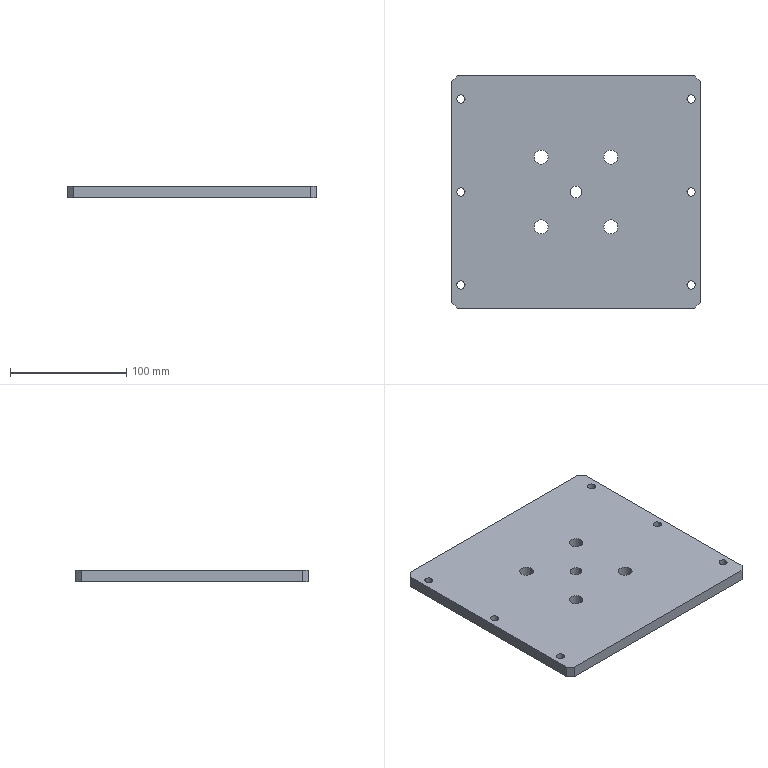Part | STEP file | Bracket upper plate | 1 solid | 32 faces | box 214 x 200 x 10 mm | volume 419850 mm3 | cylinder 22 | plane 10 | commonest cylinder face diameters 7 x12 12 x8 10.2 x2
STEP:
#1=CARTESIAN_POINT('',(-5.1,0.,0.));
#2=VERTEX_POINT('',#1);
#3=CARTESIAN_POINT('',(5.1,0.,0.));
#4=VERTEX_POINT('',#3);
#5=CARTESIAN_POINT('',(0.,0.,0.));
#6=DIRECTION('',(0.,0.,1.));
#7=DIRECTION('',(1.,0.,0.));
#8=AXIS2_PLACEMENT_3D('',#5,#6,#7);
#9=CIRCLE('',#8,5.1);
#10=EDGE_CURVE('',#2,#4,#9,.T.);
#11=ORIENTED_EDGE('',*,*,#10,.F.);
#12=CARTESIAN_POINT('',(-5.1,0.,10.));
#13=VERTEX_POINT('',#12);
#14=CARTESIAN_POINT('',(-5.1,0.,10.));
#15=DIRECTION('',(0.,0.,1.));
#16=VECTOR('',#15,1000.);
#17=LINE('',#14,#16);
#18=EDGE_CURVE('',#2,#13,#17,.T.);
#19=ORIENTED_EDGE('',*,*,#18,.T.);
#20=CARTESIAN_POINT('',(5.1,0.,10.));
#21=VERTEX_POINT('',#20);
#22=CARTESIAN_POINT('',(0.,0.,10.));
#23=DIRECTION('',(0.,0.,1.));
#24=DIRECTION('',(1.,0.,0.));
#25=AXIS2_PLACEMENT_3D('',#22,#23,#24);
#26=CIRCLE('',#25,5.1);
#27=EDGE_CURVE('',#13,#21,#26,.T.);
#28=ORIENTED_EDGE('',*,*,#27,.T.);
#29=CARTESIAN_POINT('',(5.1,0.,10.));
#30=DIRECTION('',(0.,0.,1.));
#31=VECTOR('',#30,1000.);
#32=LINE('',#29,#31);
#33=EDGE_CURVE('',#4,#21,#32,.T.);
#34=ORIENTED_EDGE('',*,*,#33,.F.);
#35=EDGE_LOOP('',(#11,#19,#28,#34));
#36=FACE_OUTER_BOUND('',#35,.T.);
#37=CARTESIAN_POINT('',(0.,0.,10.));
#38=DIRECTION('',(0.,0.,1.));
#39=DIRECTION('',(1.,0.,0.));
#40=AXIS2_PLACEMENT_3D('',#37,#38,#39);
#41=CYLINDRICAL_SURFACE('',#40,5.1);
#42=ADVANCED_FACE('',(#36),#41,.F.);
#43=CARTESIAN_POINT('',(-24.,-30.,0.));
#44=VERTEX_POINT('',#43);
#45=CARTESIAN_POINT('',(-36.,-30.,0.));
#46=VERTEX_POINT('',#45);
#47=CARTESIAN_POINT('',(-30.,-30.,0.));
#48=DIRECTION('',(0.,0.,-1.));
#49=DIRECTION('',(1.,0.,0.));
#50=AXIS2_PLACEMENT_3D('',#47,#48,#49);
#51=CIRCLE('',#50,6.);
#52=EDGE_CURVE('',#44,#46,#51,.T.);
#53=ORIENTED_EDGE('',*,*,#52,.T.);
#54=CARTESIAN_POINT('',(-36.,-30.,10.));
#55=VERTEX_POINT('',#54);
#56=CARTESIAN_POINT('',(-36.,-30.,-2.));
#57=DIRECTION('',(0.,0.,1.));
#58=VECTOR('',#57,1000.);
#59=LINE('',#56,#58);
#60=EDGE_CURVE('',#46,#55,#59,.T.);
#61=ORIENTED_EDGE('',*,*,#60,.T.);
#62=CARTESIAN_POINT('',(-24.,-30.,10.));
#63=VERTEX_POINT('',#62);
#64=CARTESIAN_POINT('',(-30.,-30.,10.));
#65=DIRECTION('',(0.,0.,-1.));
#66=DIRECTION('',(1.,0.,0.));
#67=AXIS2_PLACEMENT_3D('',#64,#65,#66);
#68=CIRCLE('',#67,6.);
#69=EDGE_CURVE('',#63,#55,#68,.T.);
#70=ORIENTED_EDGE('',*,*,#69,.F.);
#71=CARTESIAN_POINT('',(-24.,-30.,-2.));
#72=DIRECTION('',(0.,0.,1.));
#73=VECTOR('',#72,1000.);
#74=LINE('',#71,#73);
#75=EDGE_CURVE('',#44,#63,#74,.T.);
#76=ORIENTED_EDGE('',*,*,#75,.F.);
#77=EDGE_LOOP('',(#53,#61,#70,#76));
#78=FACE_OUTER_BOUND('',#77,.T.);
#79=CARTESIAN_POINT('',(-30.,-30.,-2.));
#80=DIRECTION('',(0.,0.,1.));
#81=DIRECTION('',(1.,0.,0.));
#82=AXIS2_PLACEMENT_3D('',#79,#80,#81);
#83=CYLINDRICAL_SURFACE('',#82,6.);
#84=ADVANCED_FACE('',(#78),#83,.F.);
#85=CARTESIAN_POINT('',(24.,-30.,0.));
#86=VERTEX_POINT('',#85);
#87=CARTESIAN_POINT('',(36.,-30.,0.));
#88=VERTEX_POINT('',#87);
#89=CARTESIAN_POINT('',(30.,-30.,0.));
#90=DIRECTION('',(0.,0.,1.));
#91=DIRECTION('',(1.,0.,0.));
#92=AXIS2_PLACEMENT_3D('',#89,#90,#91);
#93=CIRCLE('',#92,6.);
#94=EDGE_CURVE('',#86,#88,#93,.T.);
#95=ORIENTED_EDGE('',*,*,#94,.F.);
#96=CARTESIAN_POINT('',(24.,-30.,10.));
#97=VERTEX_POINT('',#96);
#98=CARTESIAN_POINT('',(24.,-30.,-2.));
#99=DIRECTION('',(0.,0.,1.));
#100=VECTOR('',#99,1000.);
#101=LINE('',#98,#100);
#102=EDGE_CURVE('',#86,#97,#101,.T.);
#103=ORIENTED_EDGE('',*,*,#102,.T.);
#104=CARTESIAN_POINT('',(36.,-30.,10.));
#105=VERTEX_POINT('',#104);
#106=CARTESIAN_POINT('',(30.,-30.,10.));
#107=DIRECTION('',(0.,0.,1.));
#108=DIRECTION('',(-1.,0.,0.));
#109=AXIS2_PLACEMENT_3D('',#106,#107,#108);
#110=CIRCLE('',#109,6.);
#111=EDGE_CURVE('',#97,#105,#110,.T.);
#112=ORIENTED_EDGE('',*,*,#111,.T.);
#113=CARTESIAN_POINT('',(36.,-30.,-2.));
#114=DIRECTION('',(0.,0.,1.));
#115=VECTOR('',#114,1000.);
#116=LINE('',#113,#115);
#117=EDGE_CURVE('',#88,#105,#116,.T.);
#118=ORIENTED_EDGE('',*,*,#117,.F.);
#119=EDGE_LOOP('',(#95,#103,#112,#118));
#120=FACE_OUTER_BOUND('',#119,.T.);
#121=CARTESIAN_POINT('',(30.,-30.,-2.));
#122=DIRECTION('',(0.,0.,1.));
#123=DIRECTION('',(1.,0.,0.));
#124=AXIS2_PLACEMENT_3D('',#121,#122,#123);
#125=CYLINDRICAL_SURFACE('',#124,6.);
#126=ADVANCED_FACE('',(#120),#125,.F.);
#127=CARTESIAN_POINT('',(36.,30.,0.));
#128=VERTEX_POINT('',#127);
#129=CARTESIAN_POINT('',(24.,30.,0.));
#130=VERTEX_POINT('',#129);
#131=CARTESIAN_POINT('',(30.,30.,0.));
#132=DIRECTION('',(0.,0.,-1.));
#133=DIRECTION('',(1.,0.,0.));
#134=AXIS2_PLACEMENT_3D('',#131,#132,#133);
#135=CIRCLE('',#134,6.);
#136=EDGE_CURVE('',#128,#130,#135,.T.);
#137=ORIENTED_EDGE('',*,*,#136,.T.);
#138=CARTESIAN_POINT('',(24.,30.,10.));
#139=VERTEX_POINT('',#138);
#140=CARTESIAN_POINT('',(24.,30.,-2.));
#141=DIRECTION('',(0.,0.,1.));
#142=VECTOR('',#141,1000.);
#143=LINE('',#140,#142);
#144=EDGE_CURVE('',#130,#139,#143,.T.);
#145=ORIENTED_EDGE('',*,*,#144,.T.);
#146=CARTESIAN_POINT('',(36.,30.,10.));
#147=VERTEX_POINT('',#146);
#148=CARTESIAN_POINT('',(30.,30.,10.));
#149=DIRECTION('',(0.,0.,-1.));
#150=DIRECTION('',(-1.,0.,0.));
#151=AXIS2_PLACEMENT_3D('',#148,#149,#150);
#152=CIRCLE('',#151,6.);
#153=EDGE_CURVE('',#147,#139,#152,.T.);
#154=ORIENTED_EDGE('',*,*,#153,.F.);
#155=CARTESIAN_POINT('',(36.,30.,-2.));
#156=DIRECTION('',(0.,0.,1.));
#157=VECTOR('',#156,1000.);
#158=LINE('',#155,#157);
#159=EDGE_CURVE('',#128,#147,#158,.T.);
#160=ORIENTED_EDGE('',*,*,#159,.F.);
#161=EDGE_LOOP('',(#137,#145,#154,#160));
#162=FACE_OUTER_BOUND('',#161,.T.);
#163=CARTESIAN_POINT('',(30.,30.,-2.));
#164=DIRECTION('',(0.,0.,1.));
#165=DIRECTION('',(1.,0.,0.));
#166=AXIS2_PLACEMENT_3D('',#163,#164,#165);
#167=CYLINDRICAL_SURFACE('',#166,6.);
#168=ADVANCED_FACE('',(#162),#167,.F.);
#169=CARTESIAN_POINT('',(-36.,30.,0.));
#170=VERTEX_POINT('',#169);
#171=CARTESIAN_POINT('',(-24.,30.,0.));
#172=VERTEX_POINT('',#171);
#173=CARTESIAN_POINT('',(-30.,30.,0.));
#174=DIRECTION('',(0.,0.,1.));
#175=DIRECTION('',(1.,0.,0.));
#176=AXIS2_PLACEMENT_3D('',#173,#174,#175);
#177=CIRCLE('',#176,6.);
#178=EDGE_CURVE('',#170,#172,#177,.T.);
#179=ORIENTED_EDGE('',*,*,#178,.F.);
#180=CARTESIAN_POINT('',(-36.,30.,10.));
#181=VERTEX_POINT('',#180);
#182=CARTESIAN_POINT('',(-36.,30.,-2.));
#183=DIRECTION('',(0.,0.,1.));
#184=VECTOR('',#183,1000.);
#185=LINE('',#182,#184);
#186=EDGE_CURVE('',#170,#181,#185,.T.);
#187=ORIENTED_EDGE('',*,*,#186,.T.);
#188=CARTESIAN_POINT('',(-24.,30.,10.));
#189=VERTEX_POINT('',#188);
#190=CARTESIAN_POINT('',(-30.,30.,10.));
#191=DIRECTION('',(0.,0.,1.));
#192=DIRECTION('',(1.,0.,0.));
#193=AXIS2_PLACEMENT_3D('',#190,#191,#192);
#194=CIRCLE('',#193,6.);
#195=EDGE_CURVE('',#181,#189,#194,.T.);
#196=ORIENTED_EDGE('',*,*,#195,.T.);
#197=CARTESIAN_POINT('',(-24.,30.,-2.));
#198=DIRECTION('',(0.,0.,1.));
#199=VECTOR('',#198,1000.);
#200=LINE('',#197,#199);
#201=EDGE_CURVE('',#172,#189,#200,.T.);
#202=ORIENTED_EDGE('',*,*,#201,.F.);
#203=EDGE_LOOP('',(#179,#187,#196,#202));
#204=FACE_OUTER_BOUND('',#203,.T.);
#205=CARTESIAN_POINT('',(-30.,30.,-2.));
#206=DIRECTION('',(0.,0.,1.));
#207=DIRECTION('',(1.,0.,0.));
#208=AXIS2_PLACEMENT_3D('',#205,#206,#207);
#209=CYLINDRICAL_SURFACE('',#208,6.);
#210=ADVANCED_FACE('',(#204),#209,.F.);
#211=CARTESIAN_POINT('',(102.5,0.,0.));
#212=VERTEX_POINT('',#211);
#213=CARTESIAN_POINT('',(95.5,0.,0.));
#214=VERTEX_POINT('',#213);
#215=CARTESIAN_POINT('',(99.,0.,0.));
#216=DIRECTION('',(0.,0.,-1.));
#217=DIRECTION('',(-1.,0.,0.));
#218=AXIS2_PLACEMENT_3D('',#215,#216,#217);
#219=CIRCLE('',#218,3.5);
#220=EDGE_CURVE('',#212,#214,#219,.T.);
#221=ORIENTED_EDGE('',*,*,#220,.T.);
#222=CARTESIAN_POINT('',(95.5,0.,10.));
#223=VERTEX_POINT('',#222);
#224=CARTESIAN_POINT('',(95.5,0.,0.));
#225=DIRECTION('',(0.,0.,1.));
#226=VECTOR('',#225,1000.);
#227=LINE('',#224,#226);
#228=EDGE_CURVE('',#214,#223,#227,.T.);
#229=ORIENTED_EDGE('',*,*,#228,.T.);
#230=CARTESIAN_POINT('',(102.5,0.,10.));
#231=VERTEX_POINT('',#230);
#232=CARTESIAN_POINT('',(99.,0.,10.));
#233=DIRECTION('',(0.,0.,-1.));
#234=DIRECTION('',(-1.,0.,0.));
#235=AXIS2_PLACEMENT_3D('',#232,#233,#234);
#236=CIRCLE('',#235,3.5);
#237=EDGE_CURVE('',#231,#223,#236,.T.);
#238=ORIENTED_EDGE('',*,*,#237,.F.);
#239=CARTESIAN_POINT('',(102.5,0.,0.));
#240=DIRECTION('',(0.,0.,1.));
#241=VECTOR('',#240,1000.);
#242=LINE('',#239,#241);
#243=EDGE_CURVE('',#212,#231,#242,.T.);
#244=ORIENTED_EDGE('',*,*,#243,.F.);
#245=EDGE_LOOP('',(#221,#229,#238,#244));
#246=FACE_OUTER_BOUND('',#245,.T.);
#247=CARTESIAN_POINT('',(99.,0.,0.));
#248=DIRECTION('',(0.,0.,1.));
#249=DIRECTION('',(1.,0.,0.));
#250=AXIS2_PLACEMENT_3D('',#247,#248,#249);
#251=CYLINDRICAL_SURFACE('',#250,3.5);
#252=ADVANCED_FACE('',(#246),#251,.F.);
#253=CARTESIAN_POINT('',(102.5,-80.,0.));
#254=VERTEX_POINT('',#253);
#255=CARTESIAN_POINT('',(95.5,-80.,0.));
#256=VERTEX_POINT('',#255);
#257=CARTESIAN_POINT('',(99.,-80.,0.));
#258=DIRECTION('',(0.,0.,-1.));
#259=DIRECTION('',(-1.,0.,0.));
#260=AXIS2_PLACEMENT_3D('',#257,#258,#259);
#261=CIRCLE('',#260,3.5);
#262=EDGE_CURVE('',#254,#256,#261,.T.);
#263=ORIENTED_EDGE('',*,*,#262,.T.);
#264=CARTESIAN_POINT('',(95.5,-80.,10.));
#265=VERTEX_POINT('',#264);
#266=CARTESIAN_POINT('',(95.5,-80.,0.));
#267=DIRECTION('',(0.,0.,1.));
#268=VECTOR('',#267,1000.);
#269=LINE('',#266,#268);
#270=EDGE_CURVE('',#256,#265,#269,.T.);
#271=ORIENTED_EDGE('',*,*,#270,.T.);
#272=CARTESIAN_POINT('',(102.5,-80.,10.));
#273=VERTEX_POINT('',#272);
#274=CARTESIAN_POINT('',(99.,-80.,10.));
#275=DIRECTION('',(0.,0.,-1.));
#276=DIRECTION('',(-1.,0.,0.));
#277=AXIS2_PLACEMENT_3D('',#274,#275,#276);
#278=CIRCLE('',#277,3.5);
#279=EDGE_CURVE('',#273,#265,#278,.T.);
#280=ORIENTED_EDGE('',*,*,#279,.F.);
#281=CARTESIAN_POINT('',(102.5,-80.,0.));
#282=DIRECTION('',(0.,0.,1.));
#283=VECTOR('',#282,1000.);
#284=LINE('',#281,#283);
#285=EDGE_CURVE('',#254,#273,#284,.T.);
#286=ORIENTED_EDGE('',*,*,#285,.F.);
#287=EDGE_LOOP('',(#263,#271,#280,#286));
#288=FACE_OUTER_BOUND('',#287,.T.);
#289=CARTESIAN_POINT('',(99.,-80.,0.));
#290=DIRECTION('',(0.,0.,1.));
#291=DIRECTION('',(1.,0.,0.));
#292=AXIS2_PLACEMENT_3D('',#289,#290,#291);
#293=CYLINDRICAL_SURFACE('',#292,3.5);
#294=ADVANCED_FACE('',(#288),#293,.F.);
#295=CARTESIAN_POINT('',(102.5,80.,0.));
#296=VERTEX_POINT('',#295);
#297=CARTESIAN_POINT('',(95.5,80.,0.));
#298=VERTEX_POINT('',#297);
#299=CARTESIAN_POINT('',(99.,80.,0.));
#300=DIRECTION('',(0.,0.,-1.));
#301=DIRECTION('',(-1.,0.,0.));
#302=AXIS2_PLACEMENT_3D('',#299,#300,#301);
#303=CIRCLE('',#302,3.5);
#304=EDGE_CURVE('',#296,#298,#303,.T.);
#305=ORIENTED_EDGE('',*,*,#304,.T.);
#306=CARTESIAN_POINT('',(95.5,80.,10.));
#307=VERTEX_POINT('',#306);
#308=CARTESIAN_POINT('',(95.5,80.,0.));
#309=DIRECTION('',(0.,0.,1.));
#310=VECTOR('',#309,1000.);
#311=LINE('',#308,#310);
#312=EDGE_CURVE('',#298,#307,#311,.T.);
#313=ORIENTED_EDGE('',*,*,#312,.T.);
#314=CARTESIAN_POINT('',(102.5,80.,10.));
#315=VERTEX_POINT('',#314);
#316=CARTESIAN_POINT('',(99.,80.,10.));
#317=DIRECTION('',(0.,0.,-1.));
#318=DIRECTION('',(-1.,0.,0.));
#319=AXIS2_PLACEMENT_3D('',#316,#317,#318);
#320=CIRCLE('',#319,3.5);
#321=EDGE_CURVE('',#315,#307,#320,.T.);
#322=ORIENTED_EDGE('',*,*,#321,.F.);
#323=CARTESIAN_POINT('',(102.5,80.,0.));
#324=DIRECTION('',(0.,0.,1.));
#325=VECTOR('',#324,1000.);
#326=LINE('',#323,#325);
#327=EDGE_CURVE('',#296,#315,#326,.T.);
#328=ORIENTED_EDGE('',*,*,#327,.F.);
#329=EDGE_LOOP('',(#305,#313,#322,#328));
#330=FACE_OUTER_BOUND('',#329,.T.);
#331=CARTESIAN_POINT('',(99.,80.,0.));
#332=DIRECTION('',(0.,0.,1.));
#333=DIRECTION('',(1.,0.,0.));
#334=AXIS2_PLACEMENT_3D('',#331,#332,#333);
#335=CYLINDRICAL_SURFACE('',#334,3.5);
#336=ADVANCED_FACE('',(#330),#335,.F.);
#337=CARTESIAN_POINT('',(-102.5,0.,0.));
#338=VERTEX_POINT('',#337);
#339=CARTESIAN_POINT('',(-95.5,0.,0.));
#340=VERTEX_POINT('',#339);
#341=CARTESIAN_POINT('',(-99.,0.,0.));
#342=DIRECTION('',(0.,0.,1.));
#343=DIRECTION('',(1.,0.,0.));
#344=AXIS2_PLACEMENT_3D('',#341,#342,#343);
#345=CIRCLE('',#344,3.5);
#346=EDGE_CURVE('',#338,#340,#345,.T.);
#347=ORIENTED_EDGE('',*,*,#346,.F.);
#348=CARTESIAN_POINT('',(-102.5,0.,10.));
#349=VERTEX_POINT('',#348);
#350=CARTESIAN_POINT('',(-102.5,0.,0.));
#351=DIRECTION('',(0.,0.,1.));
#352=VECTOR('',#351,1000.);
#353=LINE('',#350,#352);
#354=EDGE_CURVE('',#338,#349,#353,.T.);
#355=ORIENTED_EDGE('',*,*,#354,.T.);
#356=CARTESIAN_POINT('',(-95.5,0.,10.));
#357=VERTEX_POINT('',#356);
#358=CARTESIAN_POINT('',(-99.,0.,10.));
#359=DIRECTION('',(0.,0.,1.));
#360=DIRECTION('',(1.,0.,0.));
#361=AXIS2_PLACEMENT_3D('',#358,#359,#360);
#362=CIRCLE('',#361,3.5);
#363=EDGE_CURVE('',#349,#357,#362,.T.);
#364=ORIENTED_EDGE('',*,*,#363,.T.);
#365=CARTESIAN_POINT('',(-95.5,0.,0.));
#366=DIRECTION('',(0.,0.,1.));
#367=VECTOR('',#366,1000.);
#368=LINE('',#365,#367);
#369=EDGE_CURVE('',#340,#357,#368,.T.);
#370=ORIENTED_EDGE('',*,*,#369,.F.);
#371=EDGE_LOOP('',(#347,#355,#364,#370));
#372=FACE_OUTER_BOUND('',#371,.T.);
#373=CARTESIAN_POINT('',(-99.,0.,0.));
#374=DIRECTION('',(0.,0.,1.));
#375=DIRECTION('',(1.,0.,0.));
#376=AXIS2_PLACEMENT_3D('',#373,#374,#375);
#377=CYLINDRICAL_SURFACE('',#376,3.5);
#378=ADVANCED_FACE('',(#372),#377,.F.);
#379=CARTESIAN_POINT('',(-102.5,-80.,0.));
#380=VERTEX_POINT('',#379);
#381=CARTESIAN_POINT('',(-95.5,-80.,0.));
#382=VERTEX_POINT('',#381);
#383=CARTESIAN_POINT('',(-99.,-80.,0.));
#384=DIRECTION('',(0.,0.,1.));
#385=DIRECTION('',(1.,0.,0.));
#386=AXIS2_PLACEMENT_3D('',#383,#384,#385);
#387=CIRCLE('',#386,3.5);
#388=EDGE_CURVE('',#380,#382,#387,.T.);
#389=ORIENTED_EDGE('',*,*,#388,.F.);
#390=CARTESIAN_POINT('',(-102.5,-80.,10.));
#391=VERTEX_POINT('',#390);
#392=CARTESIAN_POINT('',(-102.5,-80.,0.));
#393=DIRECTION('',(0.,0.,1.));
#394=VECTOR('',#393,1000.);
#395=LINE('',#392,#394);
#396=EDGE_CURVE('',#380,#391,#395,.T.);
#397=ORIENTED_EDGE('',*,*,#396,.T.);
#398=CARTESIAN_POINT('',(-95.5,-80.,10.));
#399=VERTEX_POINT('',#398);
#400=CARTESIAN_POINT('',(-99.,-80.,10.));
#401=DIRECTION('',(0.,0.,1.));
#402=DIRECTION('',(1.,0.,0.));
#403=AXIS2_PLACEMENT_3D('',#400,#401,#402);
#404=CIRCLE('',#403,3.5);
#405=EDGE_CURVE('',#391,#399,#404,.T.);
#406=ORIENTED_EDGE('',*,*,#405,.T.);
#407=CARTESIAN_POINT('',(-95.5,-80.,0.));
#408=DIRECTION('',(0.,0.,1.));
#409=VECTOR('',#408,1000.);
#410=LINE('',#407,#409);
#411=EDGE_CURVE('',#382,#399,#410,.T.);
#412=ORIENTED_EDGE('',*,*,#411,.F.);
#413=EDGE_LOOP('',(#389,#397,#406,#412));
#414=FACE_OUTER_BOUND('',#413,.T.);
#415=CARTESIAN_POINT('',(-99.,-80.,0.));
#416=DIRECTION('',(0.,0.,1.));
#417=DIRECTION('',(1.,0.,0.));
#418=AXIS2_PLACEMENT_3D('',#415,#416,#417);
#419=CYLINDRICAL_SURFACE('',#418,3.5);
#420=ADVANCED_FACE('',(#414),#419,.F.);
#421=CARTESIAN_POINT('',(-102.5,80.,0.));
#422=VERTEX_POINT('',#421);
#423=CARTESIAN_POINT('',(-95.5,80.,0.));
#424=VERTEX_POINT('',#423);
#425=CARTESIAN_POINT('',(-99.,80.,0.));
#426=DIRECTION('',(0.,0.,1.));
#427=DIRECTION('',(1.,0.,0.));
#428=AXIS2_PLACEMENT_3D('',#425,#426,#427);
#429=CIRCLE('',#428,3.5);
#430=EDGE_CURVE('',#422,#424,#429,.T.);
#431=ORIENTED_EDGE('',*,*,#430,.F.);
#432=CARTESIAN_POINT('',(-102.5,80.,10.));
#433=VERTEX_POINT('',#432);
#434=CARTESIAN_POINT('',(-102.5,80.,0.));
#435=DIRECTION('',(0.,0.,1.));
#436=VECTOR('',#435,1000.);
#437=LINE('',#434,#436);
#438=EDGE_CURVE('',#422,#433,#437,.T.);
#439=ORIENTED_EDGE('',*,*,#438,.T.);
#440=CARTESIAN_POINT('',(-95.5,80.,10.));
#441=VERTEX_POINT('',#440);
#442=CARTESIAN_POINT('',(-99.,80.,10.));
#443=DIRECTION('',(0.,0.,1.));
#444=DIRECTION('',(1.,0.,0.));
#445=AXIS2_PLACEMENT_3D('',#442,#443,#444);
#446=CIRCLE('',#445,3.5);
#447=EDGE_CURVE('',#433,#441,#446,.T.);
#448=ORIENTED_EDGE('',*,*,#447,.T.);
#449=CARTESIAN_POINT('',(-95.5,80.,0.));
#450=DIRECTION('',(0.,0.,1.));
#451=VECTOR('',#450,1000.);
#452=LINE('',#449,#451);
#453=EDGE_CURVE('',#424,#441,#452,.T.);
#454=ORIENTED_EDGE('',*,*,#453,.F.);
#455=EDGE_LOOP('',(#431,#439,#448,#454));
#456=FACE_OUTER_BOUND('',#455,.T.);
#457=CARTESIAN_POINT('',(-99.,80.,0.));
#458=DIRECTION('',(0.,0.,1.));
#459=DIRECTION('',(1.,0.,0.));
#460=AXIS2_PLACEMENT_3D('',#457,#458,#459);
#461=CYLINDRICAL_SURFACE('',#460,3.5);
#462=ADVANCED_FACE('',(#456),#461,.F.);
#463=CARTESIAN_POINT('',(107.,-95.,0.));
#464=VERTEX_POINT('',#463);
#465=CARTESIAN_POINT('',(107.,95.,0.));
#466=VERTEX_POINT('',#465);
#467=CARTESIAN_POINT('',(107.,100.,0.));
#468=DIRECTION('',(0.,1.,0.));
#469=VECTOR('',#468,1000.);
#470=LINE('',#467,#469);
#471=EDGE_CURVE('',#464,#466,#470,.T.);
#472=ORIENTED_EDGE('',*,*,#471,.T.);
#473=CARTESIAN_POINT('',(107.,95.,10.));
#474=VERTEX_POINT('',#473);
#475=CARTESIAN_POINT('',(107.,95.,10.));
#476=DIRECTION('',(0.,0.,1.));
#477=VECTOR('',#476,1000.);
#478=LINE('',#475,#477);
#479=EDGE_CURVE('',#466,#474,#478,.T.);
#480=ORIENTED_EDGE('',*,*,#479,.T.);
#481=CARTESIAN_POINT('',(107.,-95.,10.));
#482=VERTEX_POINT('',#481);
#483=CARTESIAN_POINT('',(107.,100.,10.));
#484=DIRECTION('',(0.,1.,0.));
#485=VECTOR('',#484,1000.);
#486=LINE('',#483,#485);
#487=EDGE_CURVE('',#482,#474,#486,.T.);
#488=ORIENTED_EDGE('',*,*,#487,.F.);
#489=CARTESIAN_POINT('',(107.,-95.,10.));
#490=DIRECTION('',(0.,0.,-1.));
#491=VECTOR('',#490,1000.);
#492=LINE('',#489,#491);
#493=EDGE_CURVE('',#482,#464,#492,.T.);
#494=ORIENTED_EDGE('',*,*,#493,.T.);
#495=EDGE_LOOP('',(#472,#480,#488,#494));
#496=FACE_OUTER_BOUND('',#495,.T.);
#497=CARTESIAN_POINT('',(107.,100.,10.));
#498=DIRECTION('',(-1.,0.,0.));
#499=DIRECTION('',(0.,-1.,0.));
#500=AXIS2_PLACEMENT_3D('',#497,#498,#499);
#501=PLANE('',#500);
#502=ADVANCED_FACE('',(#496),#501,.F.);
#503=CARTESIAN_POINT('',(102.,100.,0.));
#504=VERTEX_POINT('',#503);
#505=CARTESIAN_POINT('',(-102.,100.,0.));
#506=VERTEX_POINT('',#505);
#507=CARTESIAN_POINT('',(-107.,100.,0.));
#508=DIRECTION('',(-1.,0.,0.));
#509=VECTOR('',#508,1000.);
#510=LINE('',#507,#509);
#511=EDGE_CURVE('',#504,#506,#510,.T.);
#512=ORIENTED_EDGE('',*,*,#511,.T.);
#513=CARTESIAN_POINT('',(-102.,100.,10.));
#514=VERTEX_POINT('',#513);
#515=CARTESIAN_POINT('',(-102.,100.,10.));
#516=DIRECTION('',(0.,0.,1.));
#517=VECTOR('',#516,1000.);
#518=LINE('',#515,#517);
#519=EDGE_CURVE('',#506,#514,#518,.T.);
#520=ORIENTED_EDGE('',*,*,#519,.T.);
#521=CARTESIAN_POINT('',(102.,100.,10.));
#522=VERTEX_POINT('',#521);
#523=CARTESIAN_POINT('',(-107.,100.,10.));
#524=DIRECTION('',(-1.,0.,0.));
#525=VECTOR('',#524,1000.);
#526=LINE('',#523,#525);
#527=EDGE_CURVE('',#522,#514,#526,.T.);
#528=ORIENTED_EDGE('',*,*,#527,.F.);
#529=CARTESIAN_POINT('',(102.,100.,10.));
#530=DIRECTION('',(0.,0.,-1.));
#531=VECTOR('',#530,1000.);
#532=LINE('',#529,#531);
#533=EDGE_CURVE('',#522,#504,#532,.T.);
#534=ORIENTED_EDGE('',*,*,#533,.T.);
#535=EDGE_LOOP('',(#512,#520,#528,#534));
#536=FACE_OUTER_BOUND('',#535,.T.);
#537=CARTESIAN_POINT('',(-107.,100.,10.));
#538=DIRECTION('',(0.,-1.,0.));
#539=DIRECTION('',(0.,0.,-1.));
#540=AXIS2_PLACEMENT_3D('',#537,#538,#539);
#541=PLANE('',#540);
#542=ADVANCED_FACE('',(#536),#541,.F.);
#543=CARTESIAN_POINT('',(-107.,95.,10.));
#544=VERTEX_POINT('',#543);
#545=CARTESIAN_POINT('',(-107.,-95.,10.));
#546=VERTEX_POINT('',#545);
#547=CARTESIAN_POINT('',(-107.,100.,10.));
#548=DIRECTION('',(0.,-1.,0.));
#549=VECTOR('',#548,1000.);
#550=LINE('',#547,#549);
#551=EDGE_CURVE('',#544,#546,#550,.T.);
#552=ORIENTED_EDGE('',*,*,#551,.F.);
#553=CARTESIAN_POINT('',(-107.,95.,0.));
#554=VERTEX_POINT('',#553);
#555=CARTESIAN_POINT('',(-107.,95.,10.));
#556=DIRECTION('',(0.,0.,-1.));
#557=VECTOR('',#556,1000.);
#558=LINE('',#555,#557);
#559=EDGE_CURVE('',#544,#554,#558,.T.);
#560=ORIENTED_EDGE('',*,*,#559,.T.);
#561=CARTESIAN_POINT('',(-107.,-95.,0.));
#562=VERTEX_POINT('',#561);
#563=CARTESIAN_POINT('',(-107.,100.,0.));
#564=DIRECTION('',(0.,-1.,0.));
#565=VECTOR('',#564,1000.);
#566=LINE('',#563,#565);
#567=EDGE_CURVE('',#554,#562,#566,.T.);
#568=ORIENTED_EDGE('',*,*,#567,.T.);
#569=CARTESIAN_POINT('',(-107.,-95.,10.));
#570=DIRECTION('',(0.,0.,1.));
#571=VECTOR('',#570,1000.);
#572=LINE('',#569,#571);
#573=EDGE_CURVE('',#562,#546,#572,.T.);
#574=ORIENTED_EDGE('',*,*,#573,.T.);
#575=EDGE_LOOP('',(#552,#560,#568,#574));
#576=FACE_OUTER_BOUND('',#575,.T.);
#577=CARTESIAN_POINT('',(-107.,100.,10.));
#578=DIRECTION('',(1.,0.,0.));
#579=DIRECTION('',(0.,1.,0.));
#580=AXIS2_PLACEMENT_3D('',#577,#578,#579);
#581=PLANE('',#580);
#582=ADVANCED_FACE('',(#576),#581,.F.);
#583=CARTESIAN_POINT('',(-102.,-100.,0.));
#584=VERTEX_POINT('',#583);
#585=CARTESIAN_POINT('',(102.,-100.,0.));
#586=VERTEX_POINT('',#585);
#587=CARTESIAN_POINT('',(-107.,-100.,0.));
#588=DIRECTION('',(1.,0.,0.));
#589=VECTOR('',#588,1000.);
#590=LINE('',#587,#589);
#591=EDGE_CURVE('',#584,#586,#590,.T.);
#592=ORIENTED_EDGE('',*,*,#591,.T.);
#593=CARTESIAN_POINT('',(102.,-100.,10.));
#594=VERTEX_POINT('',#593);
#595=CARTESIAN_POINT('',(102.,-100.,10.));
#596=DIRECTION('',(0.,0.,1.));
#597=VECTOR('',#596,1000.);
#598=LINE('',#595,#597);
#599=EDGE_CURVE('',#586,#594,#598,.T.);
#600=ORIENTED_EDGE('',*,*,#599,.T.);
#601=CARTESIAN_POINT('',(-102.,-100.,10.));
#602=VERTEX_POINT('',#601);
#603=CARTESIAN_POINT('',(-107.,-100.,10.));
#604=DIRECTION('',(1.,0.,0.));
#605=VECTOR('',#604,1000.);
#606=LINE('',#603,#605);
#607=EDGE_CURVE('',#602,#594,#606,.T.);
#608=ORIENTED_EDGE('',*,*,#607,.F.);
#609=CARTESIAN_POINT('',(-102.,-100.,10.));
#610=DIRECTION('',(0.,0.,-1.));
#611=VECTOR('',#610,1000.);
#612=LINE('',#609,#611);
#613=EDGE_CURVE('',#602,#584,#612,.T.);
#614=ORIENTED_EDGE('',*,*,#613,.T.);
#615=EDGE_LOOP('',(#592,#600,#608,#614));
#616=FACE_OUTER_BOUND('',#615,.T.);
#617=CARTESIAN_POINT('',(-107.,-100.,10.));
#618=DIRECTION('',(0.,1.,0.));
#619=DIRECTION('',(0.,0.,1.));
#620=AXIS2_PLACEMENT_3D('',#617,#618,#619);
#621=PLANE('',#620);
#622=ADVANCED_FACE('',(#616),#621,.F.);
#623=CARTESIAN_POINT('',(0.,0.,10.));
#624=DIRECTION('',(0.,0.,1.));
#625=DIRECTION('',(1.,0.,0.));
#626=AXIS2_PLACEMENT_3D('',#623,#624,#625);
#627=CIRCLE('',#626,5.1);
#628=EDGE_CURVE('',#21,#13,#627,.T.);
#629=ORIENTED_EDGE('',*,*,#628,.F.);
#630=ORIENTED_EDGE('',*,*,#27,.F.);
#631=EDGE_LOOP('',(#629,#630));
#632=FACE_BOUND('',#631,.T.);
#633=ORIENTED_EDGE('',*,*,#69,.T.);
#634=CARTESIAN_POINT('',(-30.,-30.,10.));
#635=DIRECTION('',(0.,0.,-1.));
#636=DIRECTION('',(1.,0.,0.));
#637=AXIS2_PLACEMENT_3D('',#634,#635,#636);
#638=CIRCLE('',#637,6.);
#639=EDGE_CURVE('',#55,#63,#638,.T.);
#640=ORIENTED_EDGE('',*,*,#639,.T.);
#641=EDGE_LOOP('',(#633,#640));
#642=FACE_BOUND('',#641,.T.);
#643=CARTESIAN_POINT('',(30.,-30.,10.));
#644=DIRECTION('',(0.,0.,1.));
#645=DIRECTION('',(-1.,0.,0.));
#646=AXIS2_PLACEMENT_3D('',#643,#644,#645);
#647=CIRCLE('',#646,6.);
#648=EDGE_CURVE('',#105,#97,#647,.T.);
#649=ORIENTED_EDGE('',*,*,#648,.F.);
#650=ORIENTED_EDGE('',*,*,#111,.F.);
#651=EDGE_LOOP('',(#649,#650));
#652=FACE_BOUND('',#651,.T.);
#653=ORIENTED_EDGE('',*,*,#153,.T.);
#654=CARTESIAN_POINT('',(30.,30.,10.));
#655=DIRECTION('',(0.,0.,-1.));
#656=DIRECTION('',(-1.,0.,0.));
#657=AXIS2_PLACEMENT_3D('',#654,#655,#656);
#658=CIRCLE('',#657,6.);
#659=EDGE_CURVE('',#139,#147,#658,.T.);
#660=ORIENTED_EDGE('',*,*,#659,.T.);
#661=EDGE_LOOP('',(#653,#660));
#662=FACE_BOUND('',#661,.T.);
#663=CARTESIAN_POINT('',(-30.,30.,10.));
#664=DIRECTION('',(0.,0.,1.));
#665=DIRECTION('',(1.,0.,0.));
#666=AXIS2_PLACEMENT_3D('',#663,#664,#665);
#667=CIRCLE('',#666,6.);
#668=EDGE_CURVE('',#189,#181,#667,.T.);
#669=ORIENTED_EDGE('',*,*,#668,.F.);
#670=ORIENTED_EDGE('',*,*,#195,.F.);
#671=EDGE_LOOP('',(#669,#670));
#672=FACE_BOUND('',#671,.T.);
#673=ORIENTED_EDGE('',*,*,#237,.T.);
#674=CARTESIAN_POINT('',(99.,0.,10.));
#675=DIRECTION('',(0.,0.,-1.));
#676=DIRECTION('',(-1.,0.,0.));
#677=AXIS2_PLACEMENT_3D('',#674,#675,#676);
#678=CIRCLE('',#677,3.5);
#679=EDGE_CURVE('',#223,#231,#678,.T.);
#680=ORIENTED_EDGE('',*,*,#679,.T.);
#681=EDGE_LOOP('',(#673,#680));
#682=FACE_BOUND('',#681,.T.);
#683=ORIENTED_EDGE('',*,*,#279,.T.);
#684=CARTESIAN_POINT('',(99.,-80.,10.));
#685=DIRECTION('',(0.,0.,-1.));
#686=DIRECTION('',(-1.,0.,0.));
#687=AXIS2_PLACEMENT_3D('',#684,#685,#686);
#688=CIRCLE('',#687,3.5);
#689=EDGE_CURVE('',#265,#273,#688,.T.);
#690=ORIENTED_EDGE('',*,*,#689,.T.);
#691=EDGE_LOOP('',(#683,#690));
#692=FACE_BOUND('',#691,.T.);
#693=ORIENTED_EDGE('',*,*,#321,.T.);
#694=CARTESIAN_POINT('',(99.,80.,10.));
#695=DIRECTION('',(0.,0.,-1.));
#696=DIRECTION('',(-1.,0.,0.));
#697=AXIS2_PLACEMENT_3D('',#694,#695,#696);
#698=CIRCLE('',#697,3.5);
#699=EDGE_CURVE('',#307,#315,#698,.T.);
#700=ORIENTED_EDGE('',*,*,#699,.T.);
#701=EDGE_LOOP('',(#693,#700));
#702=FACE_BOUND('',#701,.T.);
#703=CARTESIAN_POINT('',(-99.,0.,10.));
#704=DIRECTION('',(0.,0.,1.));
#705=DIRECTION('',(1.,0.,0.));
#706=AXIS2_PLACEMENT_3D('',#703,#704,#705);
#707=CIRCLE('',#706,3.5);
#708=EDGE_CURVE('',#357,#349,#707,.T.);
#709=ORIENTED_EDGE('',*,*,#708,.F.);
#710=ORIENTED_EDGE('',*,*,#363,.F.);
#711=EDGE_LOOP('',(#709,#710));
#712=FACE_BOUND('',#711,.T.);
#713=CARTESIAN_POINT('',(-99.,-80.,10.));
#714=DIRECTION('',(0.,0.,1.));
#715=DIRECTION('',(1.,0.,0.));
#716=AXIS2_PLACEMENT_3D('',#713,#714,#715);
#717=CIRCLE('',#716,3.5);
#718=EDGE_CURVE('',#399,#391,#717,.T.);
#719=ORIENTED_EDGE('',*,*,#718,.F.);
#720=ORIENTED_EDGE('',*,*,#405,.F.);
#721=EDGE_LOOP('',(#719,#720));
#722=FACE_BOUND('',#721,.T.);
#723=CARTESIAN_POINT('',(-99.,80.,10.));
#724=DIRECTION('',(0.,0.,1.));
#725=DIRECTION('',(1.,0.,0.));
#726=AXIS2_PLACEMENT_3D('',#723,#724,#725);
#727=CIRCLE('',#726,3.5);
#728=EDGE_CURVE('',#441,#433,#727,.T.);
#729=ORIENTED_EDGE('',*,*,#728,.F.);
#730=ORIENTED_EDGE('',*,*,#447,.F.);
#731=EDGE_LOOP('',(#729,#730));
#732=FACE_BOUND('',#731,.T.);
#733=ORIENTED_EDGE('',*,*,#527,.T.);
#734=CARTESIAN_POINT('',(-101.,101.,10.));
#735=DIRECTION('',(-0.7071,-0.7071,0.));
#736=VECTOR('',#735,1000.);
#737=LINE('',#734,#736);
#738=EDGE_CURVE('',#514,#544,#737,.T.);
#739=ORIENTED_EDGE('',*,*,#738,.T.);
#740=ORIENTED_EDGE('',*,*,#551,.T.);
#741=CARTESIAN_POINT('',(-101.,-101.,10.));
#742=DIRECTION('',(0.7071,-0.7071,0.));
#743=VECTOR('',#742,1000.);
#744=LINE('',#741,#743);
#745=EDGE_CURVE('',#546,#602,#744,.T.);
#746=ORIENTED_EDGE('',*,*,#745,.T.);
#747=ORIENTED_EDGE('',*,*,#607,.T.);
#748=CARTESIAN_POINT('',(101.,-101.,10.));
#749=DIRECTION('',(0.7071,0.7071,0.));
#750=VECTOR('',#749,1000.);
#751=LINE('',#748,#750);
#752=EDGE_CURVE('',#594,#482,#751,.T.);
#753=ORIENTED_EDGE('',*,*,#752,.T.);
#754=ORIENTED_EDGE('',*,*,#487,.T.);
#755=CARTESIAN_POINT('',(101.,101.,10.));
#756=DIRECTION('',(-0.7071,0.7071,0.));
#757=VECTOR('',#756,1000.);
#758=LINE('',#755,#757);
#759=EDGE_CURVE('',#474,#522,#758,.T.);
#760=ORIENTED_EDGE('',*,*,#759,.T.);
#761=EDGE_LOOP('',(#733,#739,#740,#746,#747,#753,#754,#760));
#762=FACE_OUTER_BOUND('',#761,.T.);
#763=CARTESIAN_POINT('',(0.,0.,10.));
#764=DIRECTION('',(0.,0.,1.));
#765=DIRECTION('',(1.,0.,0.));
#766=AXIS2_PLACEMENT_3D('',#763,#764,#765);
#767=PLANE('',#766);
#768=ADVANCED_FACE('',(#632,#642,#652,#662,#672,#682,#692,#702,#712,#722,#732,#762),#767,.T.);
#769=CARTESIAN_POINT('',(0.,0.,0.));
#770=DIRECTION('',(0.,0.,1.));
#771=DIRECTION('',(1.,0.,0.));
#772=AXIS2_PLACEMENT_3D('',#769,#770,#771);
#773=CIRCLE('',#772,5.1);
#774=EDGE_CURVE('',#4,#2,#773,.T.);
#775=ORIENTED_EDGE('',*,*,#774,.T.);
#776=ORIENTED_EDGE('',*,*,#10,.T.);
#777=EDGE_LOOP('',(#775,#776));
#778=FACE_BOUND('',#777,.T.);
#779=ORIENTED_EDGE('',*,*,#52,.F.);
#780=CARTESIAN_POINT('',(-30.,-30.,0.));
#781=DIRECTION('',(0.,0.,-1.));
#782=DIRECTION('',(1.,0.,0.));
#783=AXIS2_PLACEMENT_3D('',#780,#781,#782);
#784=CIRCLE('',#783,6.);
#785=EDGE_CURVE('',#46,#44,#784,.T.);
#786=ORIENTED_EDGE('',*,*,#785,.F.);
#787=EDGE_LOOP('',(#779,#786));
#788=FACE_BOUND('',#787,.T.);
#789=CARTESIAN_POINT('',(30.,-30.,0.));
#790=DIRECTION('',(0.,0.,1.));
#791=DIRECTION('',(1.,0.,0.));
#792=AXIS2_PLACEMENT_3D('',#789,#790,#791);
#793=CIRCLE('',#792,6.);
#794=EDGE_CURVE('',#88,#86,#793,.T.);
#795=ORIENTED_EDGE('',*,*,#794,.T.);
#796=ORIENTED_EDGE('',*,*,#94,.T.);
#797=EDGE_LOOP('',(#795,#796));
#798=FACE_BOUND('',#797,.T.);
#799=ORIENTED_EDGE('',*,*,#136,.F.);
#800=CARTESIAN_POINT('',(30.,30.,0.));
#801=DIRECTION('',(0.,0.,-1.));
#802=DIRECTION('',(1.,0.,0.));
#803=AXIS2_PLACEMENT_3D('',#800,#801,#802);
#804=CIRCLE('',#803,6.);
#805=EDGE_CURVE('',#130,#128,#804,.T.);
#806=ORIENTED_EDGE('',*,*,#805,.F.);
#807=EDGE_LOOP('',(#799,#806));
#808=FACE_BOUND('',#807,.T.);
#809=CARTESIAN_POINT('',(-30.,30.,0.));
#810=DIRECTION('',(0.,0.,1.));
#811=DIRECTION('',(1.,0.,0.));
#812=AXIS2_PLACEMENT_3D('',#809,#810,#811);
#813=CIRCLE('',#812,6.);
#814=EDGE_CURVE('',#172,#170,#813,.T.);
#815=ORIENTED_EDGE('',*,*,#814,.T.);
#816=ORIENTED_EDGE('',*,*,#178,.T.);
#817=EDGE_LOOP('',(#815,#816));
#818=FACE_BOUND('',#817,.T.);
#819=ORIENTED_EDGE('',*,*,#220,.F.);
#820=CARTESIAN_POINT('',(99.,0.,0.));
#821=DIRECTION('',(0.,0.,-1.));
#822=DIRECTION('',(-1.,0.,0.));
#823=AXIS2_PLACEMENT_3D('',#820,#821,#822);
#824=CIRCLE('',#823,3.5);
#825=EDGE_CURVE('',#214,#212,#824,.T.);
#826=ORIENTED_EDGE('',*,*,#825,.F.);
#827=EDGE_LOOP('',(#819,#826));
#828=FACE_BOUND('',#827,.T.);
#829=ORIENTED_EDGE('',*,*,#262,.F.);
#830=CARTESIAN_POINT('',(99.,-80.,0.));
#831=DIRECTION('',(0.,0.,-1.));
#832=DIRECTION('',(-1.,0.,0.));
#833=AXIS2_PLACEMENT_3D('',#830,#831,#832);
#834=CIRCLE('',#833,3.5);
#835=EDGE_CURVE('',#256,#254,#834,.T.);
#836=ORIENTED_EDGE('',*,*,#835,.F.);
#837=EDGE_LOOP('',(#829,#836));
#838=FACE_BOUND('',#837,.T.);
#839=ORIENTED_EDGE('',*,*,#304,.F.);
#840=CARTESIAN_POINT('',(99.,80.,0.));
#841=DIRECTION('',(0.,0.,-1.));
#842=DIRECTION('',(-1.,0.,0.));
#843=AXIS2_PLACEMENT_3D('',#840,#841,#842);
#844=CIRCLE('',#843,3.5);
#845=EDGE_CURVE('',#298,#296,#844,.T.);
#846=ORIENTED_EDGE('',*,*,#845,.F.);
#847=EDGE_LOOP('',(#839,#846));
#848=FACE_BOUND('',#847,.T.);
#849=CARTESIAN_POINT('',(-99.,0.,0.));
#850=DIRECTION('',(0.,0.,1.));
#851=DIRECTION('',(1.,0.,0.));
#852=AXIS2_PLACEMENT_3D('',#849,#850,#851);
#853=CIRCLE('',#852,3.5);
#854=EDGE_CURVE('',#340,#338,#853,.T.);
#855=ORIENTED_EDGE('',*,*,#854,.T.);
#856=ORIENTED_EDGE('',*,*,#346,.T.);
#857=EDGE_LOOP('',(#855,#856));
#858=FACE_BOUND('',#857,.T.);
#859=CARTESIAN_POINT('',(-99.,-80.,0.));
#860=DIRECTION('',(0.,0.,1.));
#861=DIRECTION('',(1.,0.,0.));
#862=AXIS2_PLACEMENT_3D('',#859,#860,#861);
#863=CIRCLE('',#862,3.5);
#864=EDGE_CURVE('',#382,#380,#863,.T.);
#865=ORIENTED_EDGE('',*,*,#864,.T.);
#866=ORIENTED_EDGE('',*,*,#388,.T.);
#867=EDGE_LOOP('',(#865,#866));
#868=FACE_BOUND('',#867,.T.);
#869=CARTESIAN_POINT('',(-99.,80.,0.));
#870=DIRECTION('',(0.,0.,1.));
#871=DIRECTION('',(1.,0.,0.));
#872=AXIS2_PLACEMENT_3D('',#869,#870,#871);
#873=CIRCLE('',#872,3.5);
#874=EDGE_CURVE('',#424,#422,#873,.T.);
#875=ORIENTED_EDGE('',*,*,#874,.T.);
#876=ORIENTED_EDGE('',*,*,#430,.T.);
#877=EDGE_LOOP('',(#875,#876));
#878=FACE_BOUND('',#877,.T.);
#879=ORIENTED_EDGE('',*,*,#567,.F.);
#880=CARTESIAN_POINT('',(-107.,95.,0.));
#881=DIRECTION('',(0.7071,0.7071,0.));
#882=VECTOR('',#881,1000.);
#883=LINE('',#880,#882);
#884=EDGE_CURVE('',#554,#506,#883,.T.);
#885=ORIENTED_EDGE('',*,*,#884,.T.);
#886=ORIENTED_EDGE('',*,*,#511,.F.);
#887=CARTESIAN_POINT('',(102.,100.,0.));
#888=DIRECTION('',(0.7071,-0.7071,0.));
#889=VECTOR('',#888,1000.);
#890=LINE('',#887,#889);
#891=EDGE_CURVE('',#504,#466,#890,.T.);
#892=ORIENTED_EDGE('',*,*,#891,.T.);
#893=ORIENTED_EDGE('',*,*,#471,.F.);
#894=CARTESIAN_POINT('',(107.,-95.,0.));
#895=DIRECTION('',(-0.7071,-0.7071,0.));
#896=VECTOR('',#895,1000.);
#897=LINE('',#894,#896);
#898=EDGE_CURVE('',#464,#586,#897,.T.);
#899=ORIENTED_EDGE('',*,*,#898,.T.);
#900=ORIENTED_EDGE('',*,*,#591,.F.);
#901=CARTESIAN_POINT('',(-102.,-100.,0.));
#902=DIRECTION('',(-0.7071,0.7071,0.));
#903=VECTOR('',#902,1000.);
#904=LINE('',#901,#903);
#905=EDGE_CURVE('',#584,#562,#904,.T.);
#906=ORIENTED_EDGE('',*,*,#905,.T.);
#907=EDGE_LOOP('',(#879,#885,#886,#892,#893,#899,#900,#906));
#908=FACE_OUTER_BOUND('',#907,.T.);
#909=CARTESIAN_POINT('',(0.,0.,0.));
#910=DIRECTION('',(0.,0.,1.));
#911=DIRECTION('',(1.,0.,0.));
#912=AXIS2_PLACEMENT_3D('',#909,#910,#911);
#913=PLANE('',#912);
#914=ADVANCED_FACE('',(#778,#788,#798,#808,#818,#828,#838,#848,#858,#868,#878,#908),#913,.F.);
#915=ORIENTED_EDGE('',*,*,#438,.F.);
#916=ORIENTED_EDGE('',*,*,#874,.F.);
#917=ORIENTED_EDGE('',*,*,#453,.T.);
#918=ORIENTED_EDGE('',*,*,#728,.T.);
#919=EDGE_LOOP('',(#915,#916,#917,#918));
#920=FACE_OUTER_BOUND('',#919,.T.);
#921=CARTESIAN_POINT('',(-99.,80.,0.));
#922=DIRECTION('',(0.,0.,1.));
#923=DIRECTION('',(1.,0.,0.));
#924=AXIS2_PLACEMENT_3D('',#921,#922,#923);
#925=CYLINDRICAL_SURFACE('',#924,3.5);
#926=ADVANCED_FACE('',(#920),#925,.F.);
#927=ORIENTED_EDGE('',*,*,#396,.F.);
#928=ORIENTED_EDGE('',*,*,#864,.F.);
#929=ORIENTED_EDGE('',*,*,#411,.T.);
#930=ORIENTED_EDGE('',*,*,#718,.T.);
#931=EDGE_LOOP('',(#927,#928,#929,#930));
#932=FACE_OUTER_BOUND('',#931,.T.);
#933=CARTESIAN_POINT('',(-99.,-80.,0.));
#934=DIRECTION('',(0.,0.,1.));
#935=DIRECTION('',(1.,0.,0.));
#936=AXIS2_PLACEMENT_3D('',#933,#934,#935);
#937=CYLINDRICAL_SURFACE('',#936,3.5);
#938=ADVANCED_FACE('',(#932),#937,.F.);
#939=ORIENTED_EDGE('',*,*,#354,.F.);
#940=ORIENTED_EDGE('',*,*,#854,.F.);
#941=ORIENTED_EDGE('',*,*,#369,.T.);
#942=ORIENTED_EDGE('',*,*,#708,.T.);
#943=EDGE_LOOP('',(#939,#940,#941,#942));
#944=FACE_OUTER_BOUND('',#943,.T.);
#945=CARTESIAN_POINT('',(-99.,0.,0.));
#946=DIRECTION('',(0.,0.,1.));
#947=DIRECTION('',(1.,0.,0.));
#948=AXIS2_PLACEMENT_3D('',#945,#946,#947);
#949=CYLINDRICAL_SURFACE('',#948,3.5);
#950=ADVANCED_FACE('',(#944),#949,.F.);
#951=ORIENTED_EDGE('',*,*,#312,.F.);
#952=ORIENTED_EDGE('',*,*,#845,.T.);
#953=ORIENTED_EDGE('',*,*,#327,.T.);
#954=ORIENTED_EDGE('',*,*,#699,.F.);
#955=EDGE_LOOP('',(#951,#952,#953,#954));
#956=FACE_OUTER_BOUND('',#955,.T.);
#957=CARTESIAN_POINT('',(99.,80.,0.));
#958=DIRECTION('',(0.,0.,1.));
#959=DIRECTION('',(1.,0.,0.));
#960=AXIS2_PLACEMENT_3D('',#957,#958,#959);
#961=CYLINDRICAL_SURFACE('',#960,3.5);
#962=ADVANCED_FACE('',(#956),#961,.F.);
#963=ORIENTED_EDGE('',*,*,#270,.F.);
#964=ORIENTED_EDGE('',*,*,#835,.T.);
#965=ORIENTED_EDGE('',*,*,#285,.T.);
#966=ORIENTED_EDGE('',*,*,#689,.F.);
#967=EDGE_LOOP('',(#963,#964,#965,#966));
#968=FACE_OUTER_BOUND('',#967,.T.);
#969=CARTESIAN_POINT('',(99.,-80.,0.));
#970=DIRECTION('',(0.,0.,1.));
#971=DIRECTION('',(1.,0.,0.));
#972=AXIS2_PLACEMENT_3D('',#969,#970,#971);
#973=CYLINDRICAL_SURFACE('',#972,3.5);
#974=ADVANCED_FACE('',(#968),#973,.F.);
#975=ORIENTED_EDGE('',*,*,#228,.F.);
#976=ORIENTED_EDGE('',*,*,#825,.T.);
#977=ORIENTED_EDGE('',*,*,#243,.T.);
#978=ORIENTED_EDGE('',*,*,#679,.F.);
#979=EDGE_LOOP('',(#975,#976,#977,#978));
#980=FACE_OUTER_BOUND('',#979,.T.);
#981=CARTESIAN_POINT('',(99.,0.,0.));
#982=DIRECTION('',(0.,0.,1.));
#983=DIRECTION('',(1.,0.,0.));
#984=AXIS2_PLACEMENT_3D('',#981,#982,#983);
#985=CYLINDRICAL_SURFACE('',#984,3.5);
#986=ADVANCED_FACE('',(#980),#985,.F.);
#987=ORIENTED_EDGE('',*,*,#186,.F.);
#988=ORIENTED_EDGE('',*,*,#814,.F.);
#989=ORIENTED_EDGE('',*,*,#201,.T.);
#990=ORIENTED_EDGE('',*,*,#668,.T.);
#991=EDGE_LOOP('',(#987,#988,#989,#990));
#992=FACE_OUTER_BOUND('',#991,.T.);
#993=CARTESIAN_POINT('',(-30.,30.,-2.));
#994=DIRECTION('',(0.,0.,1.));
#995=DIRECTION('',(1.,0.,0.));
#996=AXIS2_PLACEMENT_3D('',#993,#994,#995);
#997=CYLINDRICAL_SURFACE('',#996,6.);
#998=ADVANCED_FACE('',(#992),#997,.F.);
#999=ORIENTED_EDGE('',*,*,#144,.F.);
#1000=ORIENTED_EDGE('',*,*,#805,.T.);
#1001=ORIENTED_EDGE('',*,*,#159,.T.);
#1002=ORIENTED_EDGE('',*,*,#659,.F.);
#1003=EDGE_LOOP('',(#999,#1000,#1001,#1002));
#1004=FACE_OUTER_BOUND('',#1003,.T.);
#1005=CARTESIAN_POINT('',(30.,30.,-2.));
#1006=DIRECTION('',(0.,0.,1.));
#1007=DIRECTION('',(1.,0.,0.));
#1008=AXIS2_PLACEMENT_3D('',#1005,#1006,#1007);
#1009=CYLINDRICAL_SURFACE('',#1008,6.);
#1010=ADVANCED_FACE('',(#1004),#1009,.F.);
#1011=ORIENTED_EDGE('',*,*,#102,.F.);
#1012=ORIENTED_EDGE('',*,*,#794,.F.);
#1013=ORIENTED_EDGE('',*,*,#117,.T.);
#1014=ORIENTED_EDGE('',*,*,#648,.T.);
#1015=EDGE_LOOP('',(#1011,#1012,#1013,#1014));
#1016=FACE_OUTER_BOUND('',#1015,.T.);
#1017=CARTESIAN_POINT('',(30.,-30.,-2.));
#1018=DIRECTION('',(0.,0.,1.));
#1019=DIRECTION('',(1.,0.,0.));
#1020=AXIS2_PLACEMENT_3D('',#1017,#1018,#1019);
#1021=CYLINDRICAL_SURFACE('',#1020,6.);
#1022=ADVANCED_FACE('',(#1016),#1021,.F.);
#1023=ORIENTED_EDGE('',*,*,#60,.F.);
#1024=ORIENTED_EDGE('',*,*,#785,.T.);
#1025=ORIENTED_EDGE('',*,*,#75,.T.);
#1026=ORIENTED_EDGE('',*,*,#639,.F.);
#1027=EDGE_LOOP('',(#1023,#1024,#1025,#1026));
#1028=FACE_OUTER_BOUND('',#1027,.T.);
#1029=CARTESIAN_POINT('',(-30.,-30.,-2.));
#1030=DIRECTION('',(0.,0.,1.));
#1031=DIRECTION('',(1.,0.,0.));
#1032=AXIS2_PLACEMENT_3D('',#1029,#1030,#1031);
#1033=CYLINDRICAL_SURFACE('',#1032,6.);
#1034=ADVANCED_FACE('',(#1028),#1033,.F.);
#1035=ORIENTED_EDGE('',*,*,#18,.F.);
#1036=ORIENTED_EDGE('',*,*,#774,.F.);
#1037=ORIENTED_EDGE('',*,*,#33,.T.);
#1038=ORIENTED_EDGE('',*,*,#628,.T.);
#1039=EDGE_LOOP('',(#1035,#1036,#1037,#1038));
#1040=FACE_OUTER_BOUND('',#1039,.T.);
#1041=CARTESIAN_POINT('',(0.,0.,10.));
#1042=DIRECTION('',(0.,0.,1.));
#1043=DIRECTION('',(1.,0.,0.));
#1044=AXIS2_PLACEMENT_3D('',#1041,#1042,#1043);
#1045=CYLINDRICAL_SURFACE('',#1044,5.1);
#1046=ADVANCED_FACE('',(#1040),#1045,.F.);
#1047=ORIENTED_EDGE('',*,*,#738,.F.);
#1048=ORIENTED_EDGE('',*,*,#519,.F.);
#1049=ORIENTED_EDGE('',*,*,#884,.F.);
#1050=ORIENTED_EDGE('',*,*,#559,.F.);
#1051=EDGE_LOOP('',(#1047,#1048,#1049,#1050));
#1052=FACE_OUTER_BOUND('',#1051,.T.);
#1053=CARTESIAN_POINT('',(-107.,95.,10.));
#1054=DIRECTION('',(0.7071,-0.7071,0.));
#1055=DIRECTION('',(0.,0.,-1.));
#1056=AXIS2_PLACEMENT_3D('',#1053,#1054,#1055);
#1057=PLANE('',#1056);
#1058=ADVANCED_FACE('',(#1052),#1057,.F.);
#1059=ORIENTED_EDGE('',*,*,#759,.F.);
#1060=ORIENTED_EDGE('',*,*,#479,.F.);
#1061=ORIENTED_EDGE('',*,*,#891,.F.);
#1062=ORIENTED_EDGE('',*,*,#533,.F.);
#1063=EDGE_LOOP('',(#1059,#1060,#1061,#1062));
#1064=FACE_OUTER_BOUND('',#1063,.T.);
#1065=CARTESIAN_POINT('',(102.,100.,10.));
#1066=DIRECTION('',(-0.7071,-0.7071,0.));
#1067=DIRECTION('',(0.,0.,-1.));
#1068=AXIS2_PLACEMENT_3D('',#1065,#1066,#1067);
#1069=PLANE('',#1068);
#1070=ADVANCED_FACE('',(#1064),#1069,.F.);
#1071=ORIENTED_EDGE('',*,*,#752,.F.);
#1072=ORIENTED_EDGE('',*,*,#599,.F.);
#1073=ORIENTED_EDGE('',*,*,#898,.F.);
#1074=ORIENTED_EDGE('',*,*,#493,.F.);
#1075=EDGE_LOOP('',(#1071,#1072,#1073,#1074));
#1076=FACE_OUTER_BOUND('',#1075,.T.);
#1077=CARTESIAN_POINT('',(107.,-95.,10.));
#1078=DIRECTION('',(-0.7071,0.7071,0.));
#1079=DIRECTION('',(0.,0.,-1.));
#1080=AXIS2_PLACEMENT_3D('',#1077,#1078,#1079);
#1081=PLANE('',#1080);
#1082=ADVANCED_FACE('',(#1076),#1081,.F.);
#1083=ORIENTED_EDGE('',*,*,#745,.F.);
#1084=ORIENTED_EDGE('',*,*,#573,.F.);
#1085=ORIENTED_EDGE('',*,*,#905,.F.);
#1086=ORIENTED_EDGE('',*,*,#613,.F.);
#1087=EDGE_LOOP('',(#1083,#1084,#1085,#1086));
#1088=FACE_OUTER_BOUND('',#1087,.T.);
#1089=CARTESIAN_POINT('',(-102.,-100.,10.));
#1090=DIRECTION('',(0.7071,0.7071,0.));
#1091=DIRECTION('',(0.,0.,-1.));
#1092=AXIS2_PLACEMENT_3D('',#1089,#1090,#1091);
#1093=PLANE('',#1092);
#1094=ADVANCED_FACE('',(#1088),#1093,.F.);
#1095=CLOSED_SHELL('',(#42,#84,#126,#168,#210,#252,#294,#336,#378,#420,#462,#502,#542,#582,#622,#768,#914,#926,#938,#950,#962,#974,#986,#998,#1010,#1022,#1034,#1046,#1058,#1070,#1082,#1094));
#1096=MANIFOLD_SOLID_BREP('',#1095);
#1097=CARTESIAN_POINT('',(0.,0.,0.));
#1098=DIRECTION('',(0.,0.,1.));
#1099=DIRECTION('',(1.,0.,0.));
#1100=AXIS2_PLACEMENT_3D('',#1097,#1098,#1099);
#1101=(LENGTH_UNIT()NAMED_UNIT(*)SI_UNIT(.MILLI.,.METRE.));
#1102=UNCERTAINTY_MEASURE_WITH_UNIT(LENGTH_MEASURE(0.00001),#1101,'','');
#1103=(NAMED_UNIT(*)PLANE_ANGLE_UNIT()SI_UNIT($,.RADIAN.));
#1104=(NAMED_UNIT(*)SI_UNIT($,.STERADIAN.)SOLID_ANGLE_UNIT());
#1105=(GEOMETRIC_REPRESENTATION_CONTEXT(3)GLOBAL_UNCERTAINTY_ASSIGNED_CONTEXT((#1102))GLOBAL_UNIT_ASSIGNED_CONTEXT((#1101,#1103,#1104))REPRESENTATION_CONTEXT('',''));
#1106=ADVANCED_BREP_SHAPE_REPRESENTATION('',(#1096,#1100),#1105);